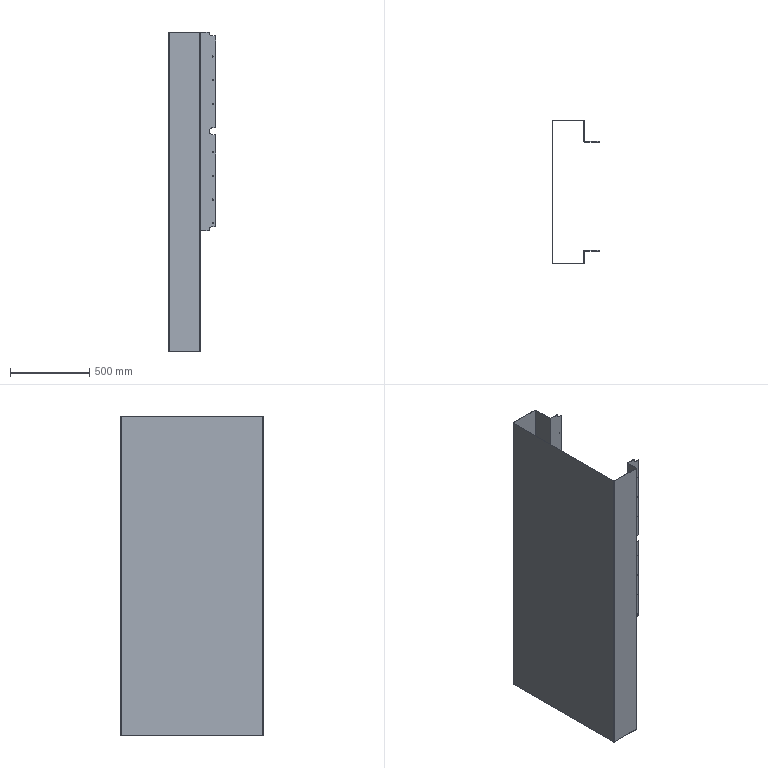Part | STEP file | C1L | 1 solid | 72 faces | box 298.717 x 900 x 2010 mm | volume 4679117 mm3 | plane 40 | cylinder 32 | commonest cylinder face diameters 7 x18 45 x6 4 x4 6 x2 10 x2